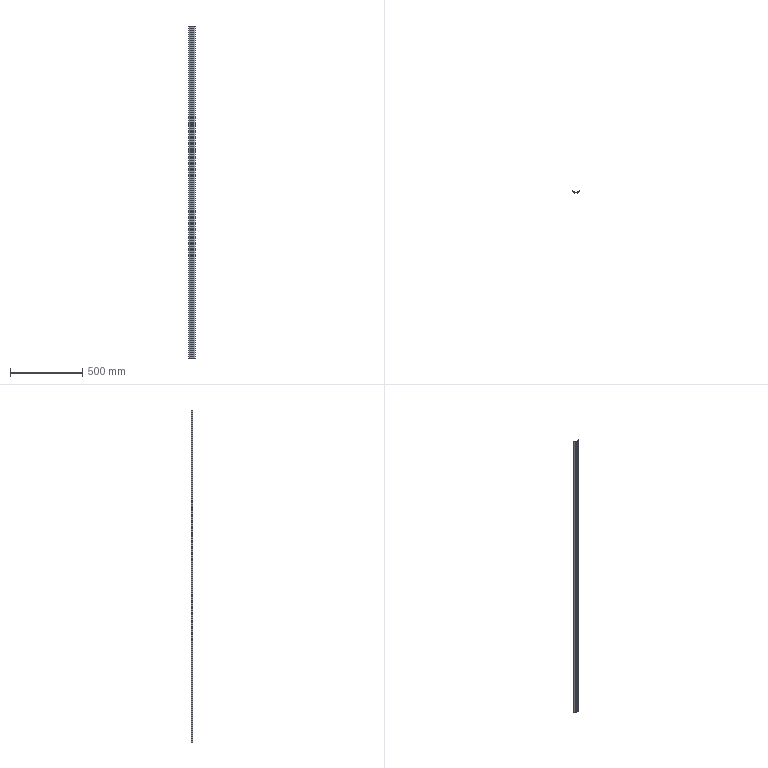Part | SolidWorks | features Extrusion 1 | 1 solid | 32 faces | box 46.782 x 13.535 x 2290 mm | volume 183913 mm3 | plane 25 | cylinder 7 | commonest cylinder face diameters 67.994 x4 0.2 x2 65.594 x1
STEP:
#1=CARTESIAN_POINT('',(-11.25,9.786,-1145.));
#2=VERTEX_POINT('',#1);
#3=CARTESIAN_POINT('',(-11.25,5.783,-1145.));
#4=VERTEX_POINT('',#3);
#5=CARTESIAN_POINT('',(-11.25,9.786,-1145.));
#6=DIRECTION('',(0.,-1.,0.));
#7=VECTOR('',#6,1000.);
#8=LINE('',#5,#7);
#9=EDGE_CURVE('',#2,#4,#8,.T.);
#10=ORIENTED_EDGE('',*,*,#9,.T.);
#11=CARTESIAN_POINT('',(-11.25,5.783,1145.));
#12=VERTEX_POINT('',#11);
#13=CARTESIAN_POINT('',(-11.25,5.783,1145.));
#14=DIRECTION('',(0.,0.,-1.));
#15=VECTOR('',#14,1000.);
#16=LINE('',#13,#15);
#17=EDGE_CURVE('',#12,#4,#16,.T.);
#18=ORIENTED_EDGE('',*,*,#17,.F.);
#19=CARTESIAN_POINT('',(-11.25,9.786,1145.));
#20=VERTEX_POINT('',#19);
#21=CARTESIAN_POINT('',(-11.25,9.786,1145.));
#22=DIRECTION('',(0.,-1.,0.));
#23=VECTOR('',#22,1000.);
#24=LINE('',#21,#23);
#25=EDGE_CURVE('',#20,#12,#24,.T.);
#26=ORIENTED_EDGE('',*,*,#25,.F.);
#27=CARTESIAN_POINT('',(-11.25,9.786,1145.));
#28=DIRECTION('',(0.,0.,-1.));
#29=VECTOR('',#28,1000.);
#30=LINE('',#27,#29);
#31=EDGE_CURVE('',#20,#2,#30,.T.);
#32=ORIENTED_EDGE('',*,*,#31,.T.);
#33=EDGE_LOOP('',(#10,#18,#26,#32));
#34=FACE_OUTER_BOUND('',#33,.T.);
#35=CARTESIAN_POINT('',(-11.25,9.786,1145.));
#36=DIRECTION('',(1.,0.,0.));
#37=DIRECTION('',(0.,0.,-1.));
#38=AXIS2_PLACEMENT_3D('',#35,#36,#37);
#39=PLANE('',#38);
#40=ADVANCED_FACE('',(#34),#39,.F.);
#41=CARTESIAN_POINT('',(-10.667,5.2,-1145.));
#42=VERTEX_POINT('',#41);
#43=CARTESIAN_POINT('',(-11.25,5.783,-1145.));
#44=DIRECTION('',(0.7071,-0.7071,0.));
#45=VECTOR('',#44,1000.);
#46=LINE('',#43,#45);
#47=EDGE_CURVE('',#4,#42,#46,.T.);
#48=ORIENTED_EDGE('',*,*,#47,.T.);
#49=CARTESIAN_POINT('',(-10.667,5.2,1145.));
#50=VERTEX_POINT('',#49);
#51=CARTESIAN_POINT('',(-10.667,5.2,1145.));
#52=DIRECTION('',(0.,0.,-1.));
#53=VECTOR('',#52,1000.);
#54=LINE('',#51,#53);
#55=EDGE_CURVE('',#50,#42,#54,.T.);
#56=ORIENTED_EDGE('',*,*,#55,.F.);
#57=CARTESIAN_POINT('',(-11.25,5.783,1145.));
#58=DIRECTION('',(0.7071,-0.7071,0.));
#59=VECTOR('',#58,1000.);
#60=LINE('',#57,#59);
#61=EDGE_CURVE('',#12,#50,#60,.T.);
#62=ORIENTED_EDGE('',*,*,#61,.F.);
#63=ORIENTED_EDGE('',*,*,#17,.T.);
#64=EDGE_LOOP('',(#48,#56,#62,#63));
#65=FACE_OUTER_BOUND('',#64,.T.);
#66=CARTESIAN_POINT('',(-11.25,5.783,1145.));
#67=DIRECTION('',(0.7071,0.7071,0.));
#68=DIRECTION('',(-0.7071,0.7071,0.));
#69=AXIS2_PLACEMENT_3D('',#66,#67,#68);
#70=PLANE('',#69);
#71=ADVANCED_FACE('',(#65),#70,.F.);
#72=CARTESIAN_POINT('',(-8.25,5.2,-1145.));
#73=VERTEX_POINT('',#72);
#74=CARTESIAN_POINT('',(-10.667,5.2,-1145.));
#75=DIRECTION('',(1.,0.,0.));
#76=VECTOR('',#75,1000.);
#77=LINE('',#74,#76);
#78=EDGE_CURVE('',#42,#73,#77,.T.);
#79=ORIENTED_EDGE('',*,*,#78,.T.);
#80=CARTESIAN_POINT('',(-8.25,5.2,1145.));
#81=VERTEX_POINT('',#80);
#82=CARTESIAN_POINT('',(-8.25,5.2,1145.));
#83=DIRECTION('',(0.,0.,-1.));
#84=VECTOR('',#83,1000.);
#85=LINE('',#82,#84);
#86=EDGE_CURVE('',#81,#73,#85,.T.);
#87=ORIENTED_EDGE('',*,*,#86,.F.);
#88=CARTESIAN_POINT('',(-10.667,5.2,1145.));
#89=DIRECTION('',(1.,0.,0.));
#90=VECTOR('',#89,1000.);
#91=LINE('',#88,#90);
#92=EDGE_CURVE('',#50,#81,#91,.T.);
#93=ORIENTED_EDGE('',*,*,#92,.F.);
#94=ORIENTED_EDGE('',*,*,#55,.T.);
#95=EDGE_LOOP('',(#79,#87,#93,#94));
#96=FACE_OUTER_BOUND('',#95,.T.);
#97=CARTESIAN_POINT('',(-10.667,5.2,1145.));
#98=DIRECTION('',(0.,1.,0.));
#99=DIRECTION('',(0.,0.,1.));
#100=AXIS2_PLACEMENT_3D('',#97,#98,#99);
#101=PLANE('',#100);
#102=ADVANCED_FACE('',(#96),#101,.F.);
#103=CARTESIAN_POINT('',(-8.25,6.,-1145.));
#104=VERTEX_POINT('',#103);
#105=CARTESIAN_POINT('',(-8.25,5.2,-1145.));
#106=DIRECTION('',(0.,1.,0.));
#107=VECTOR('',#106,1000.);
#108=LINE('',#105,#107);
#109=EDGE_CURVE('',#73,#104,#108,.T.);
#110=ORIENTED_EDGE('',*,*,#109,.T.);
#111=CARTESIAN_POINT('',(-8.25,6.,1145.));
#112=VERTEX_POINT('',#111);
#113=CARTESIAN_POINT('',(-8.25,6.,1145.));
#114=DIRECTION('',(0.,0.,-1.));
#115=VECTOR('',#114,1000.);
#116=LINE('',#113,#115);
#117=EDGE_CURVE('',#112,#104,#116,.T.);
#118=ORIENTED_EDGE('',*,*,#117,.F.);
#119=CARTESIAN_POINT('',(-8.25,5.2,1145.));
#120=DIRECTION('',(0.,1.,0.));
#121=VECTOR('',#120,1000.);
#122=LINE('',#119,#121);
#123=EDGE_CURVE('',#81,#112,#122,.T.);
#124=ORIENTED_EDGE('',*,*,#123,.F.);
#125=ORIENTED_EDGE('',*,*,#86,.T.);
#126=EDGE_LOOP('',(#110,#118,#124,#125));
#127=FACE_OUTER_BOUND('',#126,.T.);
#128=CARTESIAN_POINT('',(-8.25,5.2,1145.));
#129=DIRECTION('',(-1.,0.,0.));
#130=DIRECTION('',(0.,0.,1.));
#131=AXIS2_PLACEMENT_3D('',#128,#129,#130);
#132=PLANE('',#131);
#133=ADVANCED_FACE('',(#127),#132,.F.);
#134=CARTESIAN_POINT('',(-10.25,6.,-1145.));
#135=VERTEX_POINT('',#134);
#136=CARTESIAN_POINT('',(-8.25,6.,-1145.));
#137=DIRECTION('',(-1.,0.,0.));
#138=VECTOR('',#137,1000.);
#139=LINE('',#136,#138);
#140=EDGE_CURVE('',#104,#135,#139,.T.);
#141=ORIENTED_EDGE('',*,*,#140,.T.);
#142=CARTESIAN_POINT('',(-10.25,6.,1145.));
#143=VERTEX_POINT('',#142);
#144=CARTESIAN_POINT('',(-10.25,6.,1145.));
#145=DIRECTION('',(0.,0.,-1.));
#146=VECTOR('',#145,1000.);
#147=LINE('',#144,#146);
#148=EDGE_CURVE('',#143,#135,#147,.T.);
#149=ORIENTED_EDGE('',*,*,#148,.F.);
#150=CARTESIAN_POINT('',(-8.25,6.,1145.));
#151=DIRECTION('',(-1.,0.,0.));
#152=VECTOR('',#151,1000.);
#153=LINE('',#150,#152);
#154=EDGE_CURVE('',#112,#143,#153,.T.);
#155=ORIENTED_EDGE('',*,*,#154,.F.);
#156=ORIENTED_EDGE('',*,*,#117,.T.);
#157=EDGE_LOOP('',(#141,#149,#155,#156));
#158=FACE_OUTER_BOUND('',#157,.T.);
#159=CARTESIAN_POINT('',(-8.25,6.,1145.));
#160=DIRECTION('',(0.,-1.,0.));
#161=DIRECTION('',(0.,0.,-1.));
#162=AXIS2_PLACEMENT_3D('',#159,#160,#161);
#163=PLANE('',#162);
#164=ADVANCED_FACE('',(#158),#163,.F.);
#165=CARTESIAN_POINT('',(-10.25,7.726,-1145.));
#166=VERTEX_POINT('',#165);
#167=CARTESIAN_POINT('',(-10.25,6.,-1145.));
#168=DIRECTION('',(0.,1.,0.));
#169=VECTOR('',#168,1000.);
#170=LINE('',#167,#169);
#171=EDGE_CURVE('',#135,#166,#170,.T.);
#172=ORIENTED_EDGE('',*,*,#171,.T.);
#173=CARTESIAN_POINT('',(-10.25,7.726,1145.));
#174=VERTEX_POINT('',#173);
#175=CARTESIAN_POINT('',(-10.25,7.726,1145.));
#176=DIRECTION('',(0.,0.,-1.));
#177=VECTOR('',#176,1000.);
#178=LINE('',#175,#177);
#179=EDGE_CURVE('',#174,#166,#178,.T.);
#180=ORIENTED_EDGE('',*,*,#179,.F.);
#181=CARTESIAN_POINT('',(-10.25,6.,1145.));
#182=DIRECTION('',(0.,1.,0.));
#183=VECTOR('',#182,1000.);
#184=LINE('',#181,#183);
#185=EDGE_CURVE('',#143,#174,#184,.T.);
#186=ORIENTED_EDGE('',*,*,#185,.F.);
#187=ORIENTED_EDGE('',*,*,#148,.T.);
#188=EDGE_LOOP('',(#172,#180,#186,#187));
#189=FACE_OUTER_BOUND('',#188,.T.);
#190=CARTESIAN_POINT('',(-10.25,6.,1145.));
#191=DIRECTION('',(-1.,0.,0.));
#192=DIRECTION('',(0.,0.,1.));
#193=AXIS2_PLACEMENT_3D('',#190,#191,#192);
#194=PLANE('',#193);
#195=ADVANCED_FACE('',(#189),#194,.F.);
#196=CARTESIAN_POINT('',(-9.,7.725,-1145.));
#197=VERTEX_POINT('',#196);
#198=CARTESIAN_POINT('',(-10.25,7.726,-1145.));
#199=DIRECTION('',(1.,-0.001291,0.));
#200=VECTOR('',#199,1000.);
#201=LINE('',#198,#200);
#202=EDGE_CURVE('',#166,#197,#201,.T.);
#203=ORIENTED_EDGE('',*,*,#202,.T.);
#204=CARTESIAN_POINT('',(-9.,7.725,1145.));
#205=VERTEX_POINT('',#204);
#206=CARTESIAN_POINT('',(-9.,7.725,1145.));
#207=DIRECTION('',(0.,0.,-1.));
#208=VECTOR('',#207,1000.);
#209=LINE('',#206,#208);
#210=EDGE_CURVE('',#205,#197,#209,.T.);
#211=ORIENTED_EDGE('',*,*,#210,.F.);
#212=CARTESIAN_POINT('',(-10.25,7.726,1145.));
#213=DIRECTION('',(1.,-0.001291,0.));
#214=VECTOR('',#213,1000.);
#215=LINE('',#212,#214);
#216=EDGE_CURVE('',#174,#205,#215,.T.);
#217=ORIENTED_EDGE('',*,*,#216,.F.);
#218=ORIENTED_EDGE('',*,*,#179,.T.);
#219=EDGE_LOOP('',(#203,#211,#217,#218));
#220=FACE_OUTER_BOUND('',#219,.T.);
#221=CARTESIAN_POINT('',(-10.25,7.726,1145.));
#222=DIRECTION('',(0.001291,1.,0.));
#223=DIRECTION('',(-1.,0.001291,0.));
#224=AXIS2_PLACEMENT_3D('',#221,#222,#223);
#225=PLANE('',#224);
#226=ADVANCED_FACE('',(#220),#225,.F.);
#227=CARTESIAN_POINT('',(-8.25,8.474,-1145.));
#228=VERTEX_POINT('',#227);
#229=CARTESIAN_POINT('',(-9.,7.725,-1145.));
#230=DIRECTION('',(0.7076,0.7067,0.));
#231=VECTOR('',#230,1000.);
#232=LINE('',#229,#231);
#233=EDGE_CURVE('',#197,#228,#232,.T.);
#234=ORIENTED_EDGE('',*,*,#233,.T.);
#235=CARTESIAN_POINT('',(-8.25,8.474,1145.));
#236=VERTEX_POINT('',#235);
#237=CARTESIAN_POINT('',(-8.25,8.474,1145.));
#238=DIRECTION('',(0.,0.,-1.));
#239=VECTOR('',#238,1000.);
#240=LINE('',#237,#239);
#241=EDGE_CURVE('',#236,#228,#240,.T.);
#242=ORIENTED_EDGE('',*,*,#241,.F.);
#243=CARTESIAN_POINT('',(-9.,7.725,1145.));
#244=DIRECTION('',(0.7076,0.7067,0.));
#245=VECTOR('',#244,1000.);
#246=LINE('',#243,#245);
#247=EDGE_CURVE('',#205,#236,#246,.T.);
#248=ORIENTED_EDGE('',*,*,#247,.F.);
#249=ORIENTED_EDGE('',*,*,#210,.T.);
#250=EDGE_LOOP('',(#234,#242,#248,#249));
#251=FACE_OUTER_BOUND('',#250,.T.);
#252=CARTESIAN_POINT('',(-9.,7.725,1145.));
#253=DIRECTION('',(-0.7067,0.7076,0.));
#254=DIRECTION('',(-0.7076,-0.7067,0.));
#255=AXIS2_PLACEMENT_3D('',#252,#253,#254);
#256=PLANE('',#255);
#257=ADVANCED_FACE('',(#251),#256,.F.);
#258=CARTESIAN_POINT('',(-8.25,8.887,-1145.));
#259=VERTEX_POINT('',#258);
#260=CARTESIAN_POINT('',(-8.25,8.474,-1145.));
#261=DIRECTION('',(0.,1.,0.));
#262=VECTOR('',#261,1000.);
#263=LINE('',#260,#262);
#264=EDGE_CURVE('',#228,#259,#263,.T.);
#265=ORIENTED_EDGE('',*,*,#264,.T.);
#266=CARTESIAN_POINT('',(-8.25,8.887,1145.));
#267=VERTEX_POINT('',#266);
#268=CARTESIAN_POINT('',(-8.25,8.887,1145.));
#269=DIRECTION('',(0.,0.,-1.));
#270=VECTOR('',#269,1000.);
#271=LINE('',#268,#270);
#272=EDGE_CURVE('',#267,#259,#271,.T.);
#273=ORIENTED_EDGE('',*,*,#272,.F.);
#274=CARTESIAN_POINT('',(-8.25,8.474,1145.));
#275=DIRECTION('',(0.,1.,0.));
#276=VECTOR('',#275,1000.);
#277=LINE('',#274,#276);
#278=EDGE_CURVE('',#236,#267,#277,.T.);
#279=ORIENTED_EDGE('',*,*,#278,.F.);
#280=ORIENTED_EDGE('',*,*,#241,.T.);
#281=EDGE_LOOP('',(#265,#273,#279,#280));
#282=FACE_OUTER_BOUND('',#281,.T.);
#283=CARTESIAN_POINT('',(-8.25,8.474,1145.));
#284=DIRECTION('',(-1.,0.,0.));
#285=DIRECTION('',(0.,0.,1.));
#286=AXIS2_PLACEMENT_3D('',#283,#284,#285);
#287=PLANE('',#286);
#288=ADVANCED_FACE('',(#282),#287,.F.);
#289=CARTESIAN_POINT('',(-3.,8.003,-1145.));
#290=VERTEX_POINT('',#289);
#291=CARTESIAN_POINT('',(0.,41.867,-1145.));
#292=DIRECTION('',(0.,0.,1.));
#293=DIRECTION('',(1.,0.,0.));
#294=AXIS2_PLACEMENT_3D('',#291,#292,#293);
#295=CIRCLE('',#294,33.997);
#296=EDGE_CURVE('',#259,#290,#295,.T.);
#297=ORIENTED_EDGE('',*,*,#296,.T.);
#298=CARTESIAN_POINT('',(-3.,8.003,1145.));
#299=VERTEX_POINT('',#298);
#300=CARTESIAN_POINT('',(-3.,8.003,1145.));
#301=DIRECTION('',(0.,0.,-1.));
#302=VECTOR('',#301,1000.);
#303=LINE('',#300,#302);
#304=EDGE_CURVE('',#299,#290,#303,.T.);
#305=ORIENTED_EDGE('',*,*,#304,.F.);
#306=CARTESIAN_POINT('',(0.,41.867,1145.));
#307=DIRECTION('',(0.,0.,1.));
#308=DIRECTION('',(1.,0.,0.));
#309=AXIS2_PLACEMENT_3D('',#306,#307,#308);
#310=CIRCLE('',#309,33.997);
#311=EDGE_CURVE('',#267,#299,#310,.T.);
#312=ORIENTED_EDGE('',*,*,#311,.F.);
#313=ORIENTED_EDGE('',*,*,#272,.T.);
#314=EDGE_LOOP('',(#297,#305,#312,#313));
#315=FACE_OUTER_BOUND('',#314,.T.);
#316=CARTESIAN_POINT('',(0.,41.867,1145.));
#317=DIRECTION('',(0.,0.,-1.));
#318=DIRECTION('',(-1.,0.,0.));
#319=AXIS2_PLACEMENT_3D('',#316,#317,#318);
#320=CYLINDRICAL_SURFACE('',#319,33.997);
#321=ADVANCED_FACE('',(#315),#320,.T.);
#322=CARTESIAN_POINT('',(-3.,7.702,-1145.));
#323=VERTEX_POINT('',#322);
#324=CARTESIAN_POINT('',(-3.,8.003,-1145.));
#325=DIRECTION('',(0.,-1.,0.));
#326=VECTOR('',#325,1000.);
#327=LINE('',#324,#326);
#328=EDGE_CURVE('',#290,#323,#327,.T.);
#329=ORIENTED_EDGE('',*,*,#328,.T.);
#330=CARTESIAN_POINT('',(-3.,7.702,1145.));
#331=VERTEX_POINT('',#330);
#332=CARTESIAN_POINT('',(-3.,7.702,1145.));
#333=DIRECTION('',(0.,0.,-1.));
#334=VECTOR('',#333,1000.);
#335=LINE('',#332,#334);
#336=EDGE_CURVE('',#331,#323,#335,.T.);
#337=ORIENTED_EDGE('',*,*,#336,.F.);
#338=CARTESIAN_POINT('',(-3.,8.003,1145.));
#339=DIRECTION('',(0.,-1.,0.));
#340=VECTOR('',#339,1000.);
#341=LINE('',#338,#340);
#342=EDGE_CURVE('',#299,#331,#341,.T.);
#343=ORIENTED_EDGE('',*,*,#342,.F.);
#344=ORIENTED_EDGE('',*,*,#304,.T.);
#345=EDGE_LOOP('',(#329,#337,#343,#344));
#346=FACE_OUTER_BOUND('',#345,.T.);
#347=CARTESIAN_POINT('',(-3.,8.003,1145.));
#348=DIRECTION('',(1.,0.,0.));
#349=DIRECTION('',(0.,0.,-1.));
#350=AXIS2_PLACEMENT_3D('',#347,#348,#349);
#351=PLANE('',#350);
#352=ADVANCED_FACE('',(#346),#351,.F.);
#353=CARTESIAN_POINT('',(3.,7.702,-1145.));
#354=VERTEX_POINT('',#353);
#355=CARTESIAN_POINT('',(-3.,7.702,-1145.));
#356=DIRECTION('',(1.,0.,0.));
#357=VECTOR('',#356,1000.);
#358=LINE('',#355,#357);
#359=EDGE_CURVE('',#323,#354,#358,.T.);
#360=ORIENTED_EDGE('',*,*,#359,.T.);
#361=CARTESIAN_POINT('',(3.,7.702,1145.));
#362=VERTEX_POINT('',#361);
#363=CARTESIAN_POINT('',(3.,7.702,1145.));
#364=DIRECTION('',(0.,0.,-1.));
#365=VECTOR('',#364,1000.);
#366=LINE('',#363,#365);
#367=EDGE_CURVE('',#362,#354,#366,.T.);
#368=ORIENTED_EDGE('',*,*,#367,.F.);
#369=CARTESIAN_POINT('',(-3.,7.702,1145.));
#370=DIRECTION('',(1.,0.,0.));
#371=VECTOR('',#370,1000.);
#372=LINE('',#369,#371);
#373=EDGE_CURVE('',#331,#362,#372,.T.);
#374=ORIENTED_EDGE('',*,*,#373,.F.);
#375=ORIENTED_EDGE('',*,*,#336,.T.);
#376=EDGE_LOOP('',(#360,#368,#374,#375));
#377=FACE_OUTER_BOUND('',#376,.T.);
#378=CARTESIAN_POINT('',(-3.,7.702,1145.));
#379=DIRECTION('',(0.,1.,0.));
#380=DIRECTION('',(0.,0.,1.));
#381=AXIS2_PLACEMENT_3D('',#378,#379,#380);
#382=PLANE('',#381);
#383=ADVANCED_FACE('',(#377),#382,.F.);
#384=CARTESIAN_POINT('',(3.,8.003,-1145.));
#385=VERTEX_POINT('',#384);
#386=CARTESIAN_POINT('',(3.,7.702,-1145.));
#387=DIRECTION('',(0.,1.,0.));
#388=VECTOR('',#387,1000.);
#389=LINE('',#386,#388);
#390=EDGE_CURVE('',#354,#385,#389,.T.);
#391=ORIENTED_EDGE('',*,*,#390,.T.);
#392=CARTESIAN_POINT('',(3.,8.003,1145.));
#393=VERTEX_POINT('',#392);
#394=CARTESIAN_POINT('',(3.,8.003,1145.));
#395=DIRECTION('',(0.,0.,-1.));
#396=VECTOR('',#395,1000.);
#397=LINE('',#394,#396);
#398=EDGE_CURVE('',#393,#385,#397,.T.);
#399=ORIENTED_EDGE('',*,*,#398,.F.);
#400=CARTESIAN_POINT('',(3.,7.702,1145.));
#401=DIRECTION('',(0.,1.,0.));
#402=VECTOR('',#401,1000.);
#403=LINE('',#400,#402);
#404=EDGE_CURVE('',#362,#393,#403,.T.);
#405=ORIENTED_EDGE('',*,*,#404,.F.);
#406=ORIENTED_EDGE('',*,*,#367,.T.);
#407=EDGE_LOOP('',(#391,#399,#405,#406));
#408=FACE_OUTER_BOUND('',#407,.T.);
#409=CARTESIAN_POINT('',(3.,7.702,1145.));
#410=DIRECTION('',(-1.,0.,0.));
#411=DIRECTION('',(0.,0.,1.));
#412=AXIS2_PLACEMENT_3D('',#409,#410,#411);
#413=PLANE('',#412);
#414=ADVANCED_FACE('',(#408),#413,.F.);
#415=CARTESIAN_POINT('',(8.25,8.887,-1145.));
#416=VERTEX_POINT('',#415);
#417=CARTESIAN_POINT('',(0.,41.867,-1145.));
#418=DIRECTION('',(0.,0.,1.));
#419=DIRECTION('',(1.,0.,0.));
#420=AXIS2_PLACEMENT_3D('',#417,#418,#419);
#421=CIRCLE('',#420,33.997);
#422=EDGE_CURVE('',#385,#416,#421,.T.);
#423=ORIENTED_EDGE('',*,*,#422,.T.);
#424=CARTESIAN_POINT('',(8.25,8.887,1145.));
#425=VERTEX_POINT('',#424);
#426=CARTESIAN_POINT('',(8.25,8.887,1145.));
#427=DIRECTION('',(0.,0.,-1.));
#428=VECTOR('',#427,1000.);
#429=LINE('',#426,#428);
#430=EDGE_CURVE('',#425,#416,#429,.T.);
#431=ORIENTED_EDGE('',*,*,#430,.F.);
#432=CARTESIAN_POINT('',(0.,41.867,1145.));
#433=DIRECTION('',(0.,0.,1.));
#434=DIRECTION('',(1.,0.,0.));
#435=AXIS2_PLACEMENT_3D('',#432,#433,#434);
#436=CIRCLE('',#435,33.997);
#437=EDGE_CURVE('',#393,#425,#436,.T.);
#438=ORIENTED_EDGE('',*,*,#437,.F.);
#439=ORIENTED_EDGE('',*,*,#398,.T.);
#440=EDGE_LOOP('',(#423,#431,#438,#439));
#441=FACE_OUTER_BOUND('',#440,.T.);
#442=CARTESIAN_POINT('',(0.,41.867,1145.));
#443=DIRECTION('',(0.,0.,-1.));
#444=DIRECTION('',(-1.,0.,0.));
#445=AXIS2_PLACEMENT_3D('',#442,#443,#444);
#446=CYLINDRICAL_SURFACE('',#445,33.997);
#447=ADVANCED_FACE('',(#441),#446,.T.);
#448=CARTESIAN_POINT('',(8.25,8.474,-1145.));
#449=VERTEX_POINT('',#448);
#450=CARTESIAN_POINT('',(8.25,8.887,-1145.));
#451=DIRECTION('',(0.,-1.,0.));
#452=VECTOR('',#451,1000.);
#453=LINE('',#450,#452);
#454=EDGE_CURVE('',#416,#449,#453,.T.);
#455=ORIENTED_EDGE('',*,*,#454,.T.);
#456=CARTESIAN_POINT('',(8.25,8.474,1145.));
#457=VERTEX_POINT('',#456);
#458=CARTESIAN_POINT('',(8.25,8.474,1145.));
#459=DIRECTION('',(0.,0.,-1.));
#460=VECTOR('',#459,1000.);
#461=LINE('',#458,#460);
#462=EDGE_CURVE('',#457,#449,#461,.T.);
#463=ORIENTED_EDGE('',*,*,#462,.F.);
#464=CARTESIAN_POINT('',(8.25,8.887,1145.));
#465=DIRECTION('',(0.,-1.,0.));
#466=VECTOR('',#465,1000.);
#467=LINE('',#464,#466);
#468=EDGE_CURVE('',#425,#457,#467,.T.);
#469=ORIENTED_EDGE('',*,*,#468,.F.);
#470=ORIENTED_EDGE('',*,*,#430,.T.);
#471=EDGE_LOOP('',(#455,#463,#469,#470));
#472=FACE_OUTER_BOUND('',#471,.T.);
#473=CARTESIAN_POINT('',(8.25,8.887,1145.));
#474=DIRECTION('',(1.,0.,0.));
#475=DIRECTION('',(0.,0.,-1.));
#476=AXIS2_PLACEMENT_3D('',#473,#474,#475);
#477=PLANE('',#476);
#478=ADVANCED_FACE('',(#472),#477,.F.);
#479=CARTESIAN_POINT('',(9.,7.725,-1145.));
#480=VERTEX_POINT('',#479);
#481=CARTESIAN_POINT('',(8.25,8.474,-1145.));
#482=DIRECTION('',(0.7076,-0.7067,0.));
#483=VECTOR('',#482,1000.);
#484=LINE('',#481,#483);
#485=EDGE_CURVE('',#449,#480,#484,.T.);
#486=ORIENTED_EDGE('',*,*,#485,.T.);
#487=CARTESIAN_POINT('',(9.,7.725,1145.));
#488=VERTEX_POINT('',#487);
#489=CARTESIAN_POINT('',(9.,7.725,1145.));
#490=DIRECTION('',(0.,0.,-1.));
#491=VECTOR('',#490,1000.);
#492=LINE('',#489,#491);
#493=EDGE_CURVE('',#488,#480,#492,.T.);
#494=ORIENTED_EDGE('',*,*,#493,.F.);
#495=CARTESIAN_POINT('',(8.25,8.474,1145.));
#496=DIRECTION('',(0.7076,-0.7067,0.));
#497=VECTOR('',#496,1000.);
#498=LINE('',#495,#497);
#499=EDGE_CURVE('',#457,#488,#498,.T.);
#500=ORIENTED_EDGE('',*,*,#499,.F.);
#501=ORIENTED_EDGE('',*,*,#462,.T.);
#502=EDGE_LOOP('',(#486,#494,#500,#501));
#503=FACE_OUTER_BOUND('',#502,.T.);
#504=CARTESIAN_POINT('',(8.25,8.474,1145.));
#505=DIRECTION('',(0.7067,0.7076,0.));
#506=DIRECTION('',(-0.7076,0.7067,0.));
#507=AXIS2_PLACEMENT_3D('',#504,#505,#506);
#508=PLANE('',#507);
#509=ADVANCED_FACE('',(#503),#508,.F.);
#510=CARTESIAN_POINT('',(10.25,7.726,-1145.));
#511=VERTEX_POINT('',#510);
#512=CARTESIAN_POINT('',(9.,7.725,-1145.));
#513=DIRECTION('',(1.,0.001291,0.));
#514=VECTOR('',#513,1000.);
#515=LINE('',#512,#514);
#516=EDGE_CURVE('',#480,#511,#515,.T.);
#517=ORIENTED_EDGE('',*,*,#516,.T.);
#518=CARTESIAN_POINT('',(10.25,7.726,1145.));
#519=VERTEX_POINT('',#518);
#520=CARTESIAN_POINT('',(10.25,7.726,1145.));
#521=DIRECTION('',(0.,0.,-1.));
#522=VECTOR('',#521,1000.);
#523=LINE('',#520,#522);
#524=EDGE_CURVE('',#519,#511,#523,.T.);
#525=ORIENTED_EDGE('',*,*,#524,.F.);
#526=CARTESIAN_POINT('',(9.,7.725,1145.));
#527=DIRECTION('',(1.,0.001291,0.));
#528=VECTOR('',#527,1000.);
#529=LINE('',#526,#528);
#530=EDGE_CURVE('',#488,#519,#529,.T.);
#531=ORIENTED_EDGE('',*,*,#530,.F.);
#532=ORIENTED_EDGE('',*,*,#493,.T.);
#533=EDGE_LOOP('',(#517,#525,#531,#532));
#534=FACE_OUTER_BOUND('',#533,.T.);
#535=CARTESIAN_POINT('',(9.,7.725,1145.));
#536=DIRECTION('',(-0.001291,1.,0.));
#537=DIRECTION('',(-1.,-0.001291,0.));
#538=AXIS2_PLACEMENT_3D('',#535,#536,#537);
#539=PLANE('',#538);
#540=ADVANCED_FACE('',(#534),#539,.F.);
#541=CARTESIAN_POINT('',(10.25,6.,-1145.));
#542=VERTEX_POINT('',#541);
#543=CARTESIAN_POINT('',(10.25,7.726,-1145.));
#544=DIRECTION('',(0.,-1.,0.));
#545=VECTOR('',#544,1000.);
#546=LINE('',#543,#545);
#547=EDGE_CURVE('',#511,#542,#546,.T.);
#548=ORIENTED_EDGE('',*,*,#547,.T.);
#549=CARTESIAN_POINT('',(10.25,6.,1145.));
#550=VERTEX_POINT('',#549);
#551=CARTESIAN_POINT('',(10.25,6.,1145.));
#552=DIRECTION('',(0.,0.,-1.));
#553=VECTOR('',#552,1000.);
#554=LINE('',#551,#553);
#555=EDGE_CURVE('',#550,#542,#554,.T.);
#556=ORIENTED_EDGE('',*,*,#555,.F.);
#557=CARTESIAN_POINT('',(10.25,7.726,1145.));
#558=DIRECTION('',(0.,-1.,0.));
#559=VECTOR('',#558,1000.);
#560=LINE('',#557,#559);
#561=EDGE_CURVE('',#519,#550,#560,.T.);
#562=ORIENTED_EDGE('',*,*,#561,.F.);
#563=ORIENTED_EDGE('',*,*,#524,.T.);
#564=EDGE_LOOP('',(#548,#556,#562,#563));
#565=FACE_OUTER_BOUND('',#564,.T.);
#566=CARTESIAN_POINT('',(10.25,7.726,1145.));
#567=DIRECTION('',(1.,0.,0.));
#568=DIRECTION('',(0.,0.,-1.));
#569=AXIS2_PLACEMENT_3D('',#566,#567,#568);
#570=PLANE('',#569);
#571=ADVANCED_FACE('',(#565),#570,.F.);
#572=CARTESIAN_POINT('',(8.25,6.,-1145.));
#573=VERTEX_POINT('',#572);
#574=CARTESIAN_POINT('',(10.25,6.,-1145.));
#575=DIRECTION('',(-1.,0.,0.));
#576=VECTOR('',#575,1000.);
#577=LINE('',#574,#576);
#578=EDGE_CURVE('',#542,#573,#577,.T.);
#579=ORIENTED_EDGE('',*,*,#578,.T.);
#580=CARTESIAN_POINT('',(8.25,6.,1145.));
#581=VERTEX_POINT('',#580);
#582=CARTESIAN_POINT('',(8.25,6.,1145.));
#583=DIRECTION('',(0.,0.,-1.));
#584=VECTOR('',#583,1000.);
#585=LINE('',#582,#584);
#586=EDGE_CURVE('',#581,#573,#585,.T.);
#587=ORIENTED_EDGE('',*,*,#586,.F.);
#588=CARTESIAN_POINT('',(10.25,6.,1145.));
#589=DIRECTION('',(-1.,0.,0.));
#590=VECTOR('',#589,1000.);
#591=LINE('',#588,#590);
#592=EDGE_CURVE('',#550,#581,#591,.T.);
#593=ORIENTED_EDGE('',*,*,#592,.F.);
#594=ORIENTED_EDGE('',*,*,#555,.T.);
#595=EDGE_LOOP('',(#579,#587,#593,#594));
#596=FACE_OUTER_BOUND('',#595,.T.);
#597=CARTESIAN_POINT('',(10.25,6.,1145.));
#598=DIRECTION('',(0.,-1.,0.));
#599=DIRECTION('',(0.,0.,-1.));
#600=AXIS2_PLACEMENT_3D('',#597,#598,#599);
#601=PLANE('',#600);
#602=ADVANCED_FACE('',(#596),#601,.F.);
#603=CARTESIAN_POINT('',(8.25,5.2,-1145.));
#604=VERTEX_POINT('',#603);
#605=CARTESIAN_POINT('',(8.25,6.,-1145.));
#606=DIRECTION('',(0.,-1.,0.));
#607=VECTOR('',#606,1000.);
#608=LINE('',#605,#607);
#609=EDGE_CURVE('',#573,#604,#608,.T.);
#610=ORIENTED_EDGE('',*,*,#609,.T.);
#611=CARTESIAN_POINT('',(8.25,5.2,1145.));
#612=VERTEX_POINT('',#611);
#613=CARTESIAN_POINT('',(8.25,5.2,1145.));
#614=DIRECTION('',(0.,0.,-1.));
#615=VECTOR('',#614,1000.);
#616=LINE('',#613,#615);
#617=EDGE_CURVE('',#612,#604,#616,.T.);
#618=ORIENTED_EDGE('',*,*,#617,.F.);
#619=CARTESIAN_POINT('',(8.25,6.,1145.));
#620=DIRECTION('',(0.,-1.,0.));
#621=VECTOR('',#620,1000.);
#622=LINE('',#619,#621);
#623=EDGE_CURVE('',#581,#612,#622,.T.);
#624=ORIENTED_EDGE('',*,*,#623,.F.);
#625=ORIENTED_EDGE('',*,*,#586,.T.);
#626=EDGE_LOOP('',(#610,#618,#624,#625));
#627=FACE_OUTER_BOUND('',#626,.T.);
#628=CARTESIAN_POINT('',(8.25,6.,1145.));
#629=DIRECTION('',(1.,0.,0.));
#630=DIRECTION('',(0.,0.,-1.));
#631=AXIS2_PLACEMENT_3D('',#628,#629,#630);
#632=PLANE('',#631);
#633=ADVANCED_FACE('',(#627),#632,.F.);
#634=CARTESIAN_POINT('',(10.667,5.2,-1145.));
#635=VERTEX_POINT('',#634);
#636=CARTESIAN_POINT('',(8.25,5.2,-1145.));
#637=DIRECTION('',(1.,0.,0.));
#638=VECTOR('',#637,1000.);
#639=LINE('',#636,#638);
#640=EDGE_CURVE('',#604,#635,#639,.T.);
#641=ORIENTED_EDGE('',*,*,#640,.T.);
#642=CARTESIAN_POINT('',(10.667,5.2,1145.));
#643=VERTEX_POINT('',#642);
#644=CARTESIAN_POINT('',(10.667,5.2,1145.));
#645=DIRECTION('',(0.,0.,-1.));
#646=VECTOR('',#645,1000.);
#647=LINE('',#644,#646);
#648=EDGE_CURVE('',#643,#635,#647,.T.);
#649=ORIENTED_EDGE('',*,*,#648,.F.);
#650=CARTESIAN_POINT('',(8.25,5.2,1145.));
#651=DIRECTION('',(1.,0.,0.));
#652=VECTOR('',#651,1000.);
#653=LINE('',#650,#652);
#654=EDGE_CURVE('',#612,#643,#653,.T.);
#655=ORIENTED_EDGE('',*,*,#654,.F.);
#656=ORIENTED_EDGE('',*,*,#617,.T.);
#657=EDGE_LOOP('',(#641,#649,#655,#656));
#658=FACE_OUTER_BOUND('',#657,.T.);
#659=CARTESIAN_POINT('',(8.25,5.2,1145.));
#660=DIRECTION('',(0.,1.,0.));
#661=DIRECTION('',(0.,0.,1.));
#662=AXIS2_PLACEMENT_3D('',#659,#660,#661);
#663=PLANE('',#662);
#664=ADVANCED_FACE('',(#658),#663,.F.);
#665=CARTESIAN_POINT('',(11.25,5.783,-1145.));
#666=VERTEX_POINT('',#665);
#667=CARTESIAN_POINT('',(10.667,5.2,-1145.));
#668=DIRECTION('',(0.7071,0.7071,0.));
#669=VECTOR('',#668,1000.);
#670=LINE('',#667,#669);
#671=EDGE_CURVE('',#635,#666,#670,.T.);
#672=ORIENTED_EDGE('',*,*,#671,.T.);
#673=CARTESIAN_POINT('',(11.25,5.783,1145.));
#674=VERTEX_POINT('',#673);
#675=CARTESIAN_POINT('',(11.25,5.783,1145.));
#676=DIRECTION('',(0.,0.,-1.));
#677=VECTOR('',#676,1000.);
#678=LINE('',#675,#677);
#679=EDGE_CURVE('',#674,#666,#678,.T.);
#680=ORIENTED_EDGE('',*,*,#679,.F.);
#681=CARTESIAN_POINT('',(10.667,5.2,1145.));
#682=DIRECTION('',(0.7071,0.7071,0.));
#683=VECTOR('',#682,1000.);
#684=LINE('',#681,#683);
#685=EDGE_CURVE('',#643,#674,#684,.T.);
#686=ORIENTED_EDGE('',*,*,#685,.F.);
#687=ORIENTED_EDGE('',*,*,#648,.T.);
#688=EDGE_LOOP('',(#672,#680,#686,#687));
#689=FACE_OUTER_BOUND('',#688,.T.);
#690=CARTESIAN_POINT('',(10.667,5.2,1145.));
#691=DIRECTION('',(-0.7071,0.7071,0.));
#692=DIRECTION('',(-0.7071,-0.7071,0.));
#693=AXIS2_PLACEMENT_3D('',#690,#691,#692);
#694=PLANE('',#693);
#695=ADVANCED_FACE('',(#689),#694,.F.);
#696=CARTESIAN_POINT('',(11.25,9.786,-1145.));
#697=VERTEX_POINT('',#696);
#698=CARTESIAN_POINT('',(11.25,5.783,-1145.));
#699=DIRECTION('',(0.,1.,0.));
#700=VECTOR('',#699,1000.);
#701=LINE('',#698,#700);
#702=EDGE_CURVE('',#666,#697,#701,.T.);
#703=ORIENTED_EDGE('',*,*,#702,.T.);
#704=CARTESIAN_POINT('',(11.25,9.786,1145.));
#705=VERTEX_POINT('',#704);
#706=CARTESIAN_POINT('',(11.25,9.786,1145.));
#707=DIRECTION('',(0.,0.,-1.));
#708=VECTOR('',#707,1000.);
#709=LINE('',#706,#708);
#710=EDGE_CURVE('',#705,#697,#709,.T.);
#711=ORIENTED_EDGE('',*,*,#710,.F.);
#712=CARTESIAN_POINT('',(11.25,5.783,1145.));
#713=DIRECTION('',(0.,1.,0.));
#714=VECTOR('',#713,1000.);
#715=LINE('',#712,#714);
#716=EDGE_CURVE('',#674,#705,#715,.T.);
#717=ORIENTED_EDGE('',*,*,#716,.F.);
#718=ORIENTED_EDGE('',*,*,#679,.T.);
#719=EDGE_LOOP('',(#703,#711,#717,#718));
#720=FACE_OUTER_BOUND('',#719,.T.);
#721=CARTESIAN_POINT('',(11.25,5.783,1145.));
#722=DIRECTION('',(-1.,0.,0.));
#723=DIRECTION('',(0.,0.,1.));
#724=AXIS2_PLACEMENT_3D('',#721,#722,#723);
#725=PLANE('',#724);
#726=ADVANCED_FACE('',(#720),#725,.F.);
#727=CARTESIAN_POINT('',(23.391,17.196,-1145.));
#728=VERTEX_POINT('',#727);
#729=CARTESIAN_POINT('',(0.,41.867,-1145.));
#730=DIRECTION('',(0.,0.,1.));
#731=DIRECTION('',(1.,0.,0.));
#732=AXIS2_PLACEMENT_3D('',#729,#730,#731);
#733=CIRCLE('',#732,33.997);
#734=EDGE_CURVE('',#697,#728,#733,.T.);
#735=ORIENTED_EDGE('',*,*,#734,.T.);
#736=CARTESIAN_POINT('',(23.391,17.196,1145.));
#737=VERTEX_POINT('',#736);
#738=CARTESIAN_POINT('',(23.391,17.196,1145.));
#739=DIRECTION('',(0.,0.,-1.));
#740=VECTOR('',#739,1000.);
#741=LINE('',#738,#740);
#742=EDGE_CURVE('',#737,#728,#741,.T.);
#743=ORIENTED_EDGE('',*,*,#742,.F.);
#744=CARTESIAN_POINT('',(0.,41.867,1145.));
#745=DIRECTION('',(0.,0.,1.));
#746=DIRECTION('',(1.,0.,0.));
#747=AXIS2_PLACEMENT_3D('',#744,#745,#746);
#748=CIRCLE('',#747,33.997);
#749=EDGE_CURVE('',#705,#737,#748,.T.);
#750=ORIENTED_EDGE('',*,*,#749,.F.);
#751=ORIENTED_EDGE('',*,*,#710,.T.);
#752=EDGE_LOOP('',(#735,#743,#750,#751));
#753=FACE_OUTER_BOUND('',#752,.T.);
#754=CARTESIAN_POINT('',(0.,41.867,1145.));
#755=DIRECTION('',(0.,0.,-1.));
#756=DIRECTION('',(-1.,0.,0.));
#757=AXIS2_PLACEMENT_3D('',#754,#755,#756);
#758=CYLINDRICAL_SURFACE('',#757,33.997);
#759=ADVANCED_FACE('',(#753),#758,.T.);
#760=CARTESIAN_POINT('',(23.391,18.635,-1145.));
#761=VERTEX_POINT('',#760);
#762=CARTESIAN_POINT('',(23.391,17.196,-1145.));
#763=DIRECTION('',(0.,1.,0.));
#764=VECTOR('',#763,1000.);
#765=LINE('',#762,#764);
#766=EDGE_CURVE('',#728,#761,#765,.T.);
#767=ORIENTED_EDGE('',*,*,#766,.T.);
#768=CARTESIAN_POINT('',(23.391,18.635,1145.));
#769=VERTEX_POINT('',#768);
#770=CARTESIAN_POINT('',(23.391,18.635,1145.));
#771=DIRECTION('',(0.,0.,-1.));
#772=VECTOR('',#771,1000.);
#773=LINE('',#770,#772);
#774=EDGE_CURVE('',#769,#761,#773,.T.);
#775=ORIENTED_EDGE('',*,*,#774,.F.);
#776=CARTESIAN_POINT('',(23.391,17.196,1145.));
#777=DIRECTION('',(0.,1.,0.));
#778=VECTOR('',#777,1000.);
#779=LINE('',#776,#778);
#780=EDGE_CURVE('',#737,#769,#779,.T.);
#781=ORIENTED_EDGE('',*,*,#780,.F.);
#782=ORIENTED_EDGE('',*,*,#742,.T.);
#783=EDGE_LOOP('',(#767,#775,#781,#782));
#784=FACE_OUTER_BOUND('',#783,.T.);
#785=CARTESIAN_POINT('',(23.391,17.196,1145.));
#786=DIRECTION('',(-1.,0.,0.));
#787=DIRECTION('',(0.,0.,1.));
#788=AXIS2_PLACEMENT_3D('',#785,#786,#787);
#789=PLANE('',#788);
#790=ADVANCED_FACE('',(#784),#789,.F.);
#791=CARTESIAN_POINT('',(23.22,18.706,-1145.));
#792=VERTEX_POINT('',#791);
#793=CARTESIAN_POINT('',(23.291,18.635,-1145.));
#794=DIRECTION('',(0.,0.,1.));
#795=DIRECTION('',(1.,0.,0.));
#796=AXIS2_PLACEMENT_3D('',#793,#794,#795);
#797=CIRCLE('',#796,0.1);
#798=EDGE_CURVE('',#761,#792,#797,.T.);
#799=ORIENTED_EDGE('',*,*,#798,.T.);
#800=CARTESIAN_POINT('',(23.22,18.706,1145.));
#801=VERTEX_POINT('',#800);
#802=CARTESIAN_POINT('',(23.22,18.706,1145.));
#803=DIRECTION('',(0.,0.,-1.));
#804=VECTOR('',#803,1000.);
#805=LINE('',#802,#804);
#806=EDGE_CURVE('',#801,#792,#805,.T.);
#807=ORIENTED_EDGE('',*,*,#806,.F.);
#808=CARTESIAN_POINT('',(23.291,18.635,1145.));
#809=DIRECTION('',(0.,0.,1.));
#810=DIRECTION('',(1.,0.,0.));
#811=AXIS2_PLACEMENT_3D('',#808,#809,#810);
#812=CIRCLE('',#811,0.1);
#813=EDGE_CURVE('',#769,#801,#812,.T.);
#814=ORIENTED_EDGE('',*,*,#813,.F.);
#815=ORIENTED_EDGE('',*,*,#774,.T.);
#816=EDGE_LOOP('',(#799,#807,#814,#815));
#817=FACE_OUTER_BOUND('',#816,.T.);
#818=CARTESIAN_POINT('',(23.291,18.635,1145.));
#819=DIRECTION('',(0.,0.,-1.));
#820=DIRECTION('',(-1.,0.,0.));
#821=AXIS2_PLACEMENT_3D('',#818,#819,#820);
#822=CYLINDRICAL_SURFACE('',#821,0.1);
#823=ADVANCED_FACE('',(#817),#822,.T.);
#824=CARTESIAN_POINT('',(-23.22,18.706,-1145.));
#825=VERTEX_POINT('',#824);
#826=CARTESIAN_POINT('',(0.,41.867,-1145.));
#827=DIRECTION('',(0.,0.,-1.));
#828=DIRECTION('',(1.,0.,0.));
#829=AXIS2_PLACEMENT_3D('',#826,#827,#828);
#830=CIRCLE('',#829,32.797);
#831=EDGE_CURVE('',#792,#825,#830,.T.);
#832=ORIENTED_EDGE('',*,*,#831,.T.);
#833=CARTESIAN_POINT('',(-23.22,18.706,1145.));
#834=VERTEX_POINT('',#833);
#835=CARTESIAN_POINT('',(-23.22,18.706,1145.));
#836=DIRECTION('',(0.,0.,-1.));
#837=VECTOR('',#836,1000.);
#838=LINE('',#835,#837);
#839=EDGE_CURVE('',#834,#825,#838,.T.);
#840=ORIENTED_EDGE('',*,*,#839,.F.);
#841=CARTESIAN_POINT('',(0.,41.867,1145.));
#842=DIRECTION('',(0.,0.,-1.));
#843=DIRECTION('',(1.,0.,0.));
#844=AXIS2_PLACEMENT_3D('',#841,#842,#843);
#845=CIRCLE('',#844,32.797);
#846=EDGE_CURVE('',#801,#834,#845,.T.);
#847=ORIENTED_EDGE('',*,*,#846,.F.);
#848=ORIENTED_EDGE('',*,*,#806,.T.);
#849=EDGE_LOOP('',(#832,#840,#847,#848));
#850=FACE_OUTER_BOUND('',#849,.T.);
#851=CARTESIAN_POINT('',(0.,41.867,1145.));
#852=DIRECTION('',(0.,0.,-1.));
#853=DIRECTION('',(-1.,0.,0.));
#854=AXIS2_PLACEMENT_3D('',#851,#852,#853);
#855=CYLINDRICAL_SURFACE('',#854,32.797);
#856=ADVANCED_FACE('',(#850),#855,.F.);
#857=CARTESIAN_POINT('',(-23.391,18.635,-1145.));
#858=VERTEX_POINT('',#857);
#859=CARTESIAN_POINT('',(-23.291,18.635,-1145.));
#860=DIRECTION('',(0.,0.,1.));
#861=DIRECTION('',(1.,0.,0.));
#862=AXIS2_PLACEMENT_3D('',#859,#860,#861);
#863=CIRCLE('',#862,0.1);
#864=EDGE_CURVE('',#825,#858,#863,.T.);
#865=ORIENTED_EDGE('',*,*,#864,.T.);
#866=CARTESIAN_POINT('',(-23.391,18.635,1145.));
#867=VERTEX_POINT('',#866);
#868=CARTESIAN_POINT('',(-23.391,18.635,1145.));
#869=DIRECTION('',(0.,0.,-1.));
#870=VECTOR('',#869,1000.);
#871=LINE('',#868,#870);
#872=EDGE_CURVE('',#867,#858,#871,.T.);
#873=ORIENTED_EDGE('',*,*,#872,.F.);
#874=CARTESIAN_POINT('',(-23.291,18.635,1145.));
#875=DIRECTION('',(0.,0.,1.));
#876=DIRECTION('',(1.,0.,0.));
#877=AXIS2_PLACEMENT_3D('',#874,#875,#876);
#878=CIRCLE('',#877,0.1);
#879=EDGE_CURVE('',#834,#867,#878,.T.);
#880=ORIENTED_EDGE('',*,*,#879,.F.);
#881=ORIENTED_EDGE('',*,*,#839,.T.);
#882=EDGE_LOOP('',(#865,#873,#880,#881));
#883=FACE_OUTER_BOUND('',#882,.T.);
#884=CARTESIAN_POINT('',(-23.291,18.635,1145.));
#885=DIRECTION('',(0.,0.,-1.));
#886=DIRECTION('',(-1.,0.,0.));
#887=AXIS2_PLACEMENT_3D('',#884,#885,#886);
#888=CYLINDRICAL_SURFACE('',#887,0.1);
#889=ADVANCED_FACE('',(#883),#888,.T.);
#890=CARTESIAN_POINT('',(-23.391,17.196,-1145.));
#891=VERTEX_POINT('',#890);
#892=CARTESIAN_POINT('',(-23.391,18.635,-1145.));
#893=DIRECTION('',(0.,-1.,0.));
#894=VECTOR('',#893,1000.);
#895=LINE('',#892,#894);
#896=EDGE_CURVE('',#858,#891,#895,.T.);
#897=ORIENTED_EDGE('',*,*,#896,.T.);
#898=CARTESIAN_POINT('',(-23.391,17.196,1145.));
#899=VERTEX_POINT('',#898);
#900=CARTESIAN_POINT('',(-23.391,17.196,1145.));
#901=DIRECTION('',(0.,0.,-1.));
#902=VECTOR('',#901,1000.);
#903=LINE('',#900,#902);
#904=EDGE_CURVE('',#899,#891,#903,.T.);
#905=ORIENTED_EDGE('',*,*,#904,.F.);
#906=CARTESIAN_POINT('',(-23.391,18.635,1145.));
#907=DIRECTION('',(0.,-1.,0.));
#908=VECTOR('',#907,1000.);
#909=LINE('',#906,#908);
#910=EDGE_CURVE('',#867,#899,#909,.T.);
#911=ORIENTED_EDGE('',*,*,#910,.F.);
#912=ORIENTED_EDGE('',*,*,#872,.T.);
#913=EDGE_LOOP('',(#897,#905,#911,#912));
#914=FACE_OUTER_BOUND('',#913,.T.);
#915=CARTESIAN_POINT('',(-23.391,18.635,1145.));
#916=DIRECTION('',(1.,0.,0.));
#917=DIRECTION('',(0.,0.,-1.));
#918=AXIS2_PLACEMENT_3D('',#915,#916,#917);
#919=PLANE('',#918);
#920=ADVANCED_FACE('',(#914),#919,.F.);
#921=CARTESIAN_POINT('',(0.,41.867,-1145.));
#922=DIRECTION('',(0.,0.,1.));
#923=DIRECTION('',(1.,0.,0.));
#924=AXIS2_PLACEMENT_3D('',#921,#922,#923);
#925=CIRCLE('',#924,33.997);
#926=EDGE_CURVE('',#891,#2,#925,.T.);
#927=ORIENTED_EDGE('',*,*,#926,.T.);
#928=ORIENTED_EDGE('',*,*,#31,.F.);
#929=CARTESIAN_POINT('',(0.,41.867,1145.));
#930=DIRECTION('',(0.,0.,1.));
#931=DIRECTION('',(1.,0.,0.));
#932=AXIS2_PLACEMENT_3D('',#929,#930,#931);
#933=CIRCLE('',#932,33.997);
#934=EDGE_CURVE('',#899,#20,#933,.T.);
#935=ORIENTED_EDGE('',*,*,#934,.F.);
#936=ORIENTED_EDGE('',*,*,#904,.T.);
#937=EDGE_LOOP('',(#927,#928,#935,#936));
#938=FACE_OUTER_BOUND('',#937,.T.);
#939=CARTESIAN_POINT('',(0.,41.867,1145.));
#940=DIRECTION('',(0.,0.,-1.));
#941=DIRECTION('',(-1.,0.,0.));
#942=AXIS2_PLACEMENT_3D('',#939,#940,#941);
#943=CYLINDRICAL_SURFACE('',#942,33.997);
#944=ADVANCED_FACE('',(#938),#943,.T.);
#945=ORIENTED_EDGE('',*,*,#25,.T.);
#946=ORIENTED_EDGE('',*,*,#61,.T.);
#947=ORIENTED_EDGE('',*,*,#92,.T.);
#948=ORIENTED_EDGE('',*,*,#123,.T.);
#949=ORIENTED_EDGE('',*,*,#154,.T.);
#950=ORIENTED_EDGE('',*,*,#185,.T.);
#951=ORIENTED_EDGE('',*,*,#216,.T.);
#952=ORIENTED_EDGE('',*,*,#247,.T.);
#953=ORIENTED_EDGE('',*,*,#278,.T.);
#954=ORIENTED_EDGE('',*,*,#311,.T.);
#955=ORIENTED_EDGE('',*,*,#342,.T.);
#956=ORIENTED_EDGE('',*,*,#373,.T.);
#957=ORIENTED_EDGE('',*,*,#404,.T.);
#958=ORIENTED_EDGE('',*,*,#437,.T.);
#959=ORIENTED_EDGE('',*,*,#468,.T.);
#960=ORIENTED_EDGE('',*,*,#499,.T.);
#961=ORIENTED_EDGE('',*,*,#530,.T.);
#962=ORIENTED_EDGE('',*,*,#561,.T.);
#963=ORIENTED_EDGE('',*,*,#592,.T.);
#964=ORIENTED_EDGE('',*,*,#623,.T.);
#965=ORIENTED_EDGE('',*,*,#654,.T.);
#966=ORIENTED_EDGE('',*,*,#685,.T.);
#967=ORIENTED_EDGE('',*,*,#716,.T.);
#968=ORIENTED_EDGE('',*,*,#749,.T.);
#969=ORIENTED_EDGE('',*,*,#780,.T.);
#970=ORIENTED_EDGE('',*,*,#813,.T.);
#971=ORIENTED_EDGE('',*,*,#846,.T.);
#972=ORIENTED_EDGE('',*,*,#879,.T.);
#973=ORIENTED_EDGE('',*,*,#910,.T.);
#974=ORIENTED_EDGE('',*,*,#934,.T.);
#975=EDGE_LOOP('',(#945,#946,#947,#948,#949,#950,#951,#952,#953,#954,#955,#956,#957,#958,#959,#960,#961,#962,#963,#964,#965,#966,#967,#968,#969,#970,#971,#972,#973,#974));
#976=FACE_OUTER_BOUND('',#975,.T.);
#977=CARTESIAN_POINT('',(0.,41.867,1145.));
#978=DIRECTION('',(0.,0.,1.));
#979=DIRECTION('',(1.,0.,0.));
#980=AXIS2_PLACEMENT_3D('',#977,#978,#979);
#981=PLANE('',#980);
#982=ADVANCED_FACE('',(#976),#981,.T.);
#983=ORIENTED_EDGE('',*,*,#9,.F.);
#984=ORIENTED_EDGE('',*,*,#926,.F.);
#985=ORIENTED_EDGE('',*,*,#896,.F.);
#986=ORIENTED_EDGE('',*,*,#864,.F.);
#987=ORIENTED_EDGE('',*,*,#831,.F.);
#988=ORIENTED_EDGE('',*,*,#798,.F.);
#989=ORIENTED_EDGE('',*,*,#766,.F.);
#990=ORIENTED_EDGE('',*,*,#734,.F.);
#991=ORIENTED_EDGE('',*,*,#702,.F.);
#992=ORIENTED_EDGE('',*,*,#671,.F.);
#993=ORIENTED_EDGE('',*,*,#640,.F.);
#994=ORIENTED_EDGE('',*,*,#609,.F.);
#995=ORIENTED_EDGE('',*,*,#578,.F.);
#996=ORIENTED_EDGE('',*,*,#547,.F.);
#997=ORIENTED_EDGE('',*,*,#516,.F.);
#998=ORIENTED_EDGE('',*,*,#485,.F.);
#999=ORIENTED_EDGE('',*,*,#454,.F.);
#1000=ORIENTED_EDGE('',*,*,#422,.F.);
#1001=ORIENTED_EDGE('',*,*,#390,.F.);
#1002=ORIENTED_EDGE('',*,*,#359,.F.);
#1003=ORIENTED_EDGE('',*,*,#328,.F.);
#1004=ORIENTED_EDGE('',*,*,#296,.F.);
#1005=ORIENTED_EDGE('',*,*,#264,.F.);
#1006=ORIENTED_EDGE('',*,*,#233,.F.);
#1007=ORIENTED_EDGE('',*,*,#202,.F.);
#1008=ORIENTED_EDGE('',*,*,#171,.F.);
#1009=ORIENTED_EDGE('',*,*,#140,.F.);
#1010=ORIENTED_EDGE('',*,*,#109,.F.);
#1011=ORIENTED_EDGE('',*,*,#78,.F.);
#1012=ORIENTED_EDGE('',*,*,#47,.F.);
#1013=EDGE_LOOP('',(#983,#984,#985,#986,#987,#988,#989,#990,#991,#992,#993,#994,#995,#996,#997,#998,#999,#1000,#1001,#1002,#1003,#1004,#1005,#1006,#1007,#1008,#1009,#1010,#1011,#1012));
#1014=FACE_OUTER_BOUND('',#1013,.T.);
#1015=CARTESIAN_POINT('',(0.,41.867,-1145.));
#1016=DIRECTION('',(0.,0.,1.));
#1017=DIRECTION('',(1.,0.,0.));
#1018=AXIS2_PLACEMENT_3D('',#1015,#1016,#1017);
#1019=PLANE('',#1018);
#1020=ADVANCED_FACE('',(#1014),#1019,.F.);
#1021=CLOSED_SHELL('',(#40,#71,#102,#133,#164,#195,#226,#257,#288,#321,#352,#383,#414,#447,#478,#509,#540,#571,#602,#633,#664,#695,#726,#759,#790,#823,#856,#889,#920,#944,#982,#1020));
#1022=MANIFOLD_SOLID_BREP('',#1021);
#1023=CARTESIAN_POINT('',(0.,0.,0.));
#1024=DIRECTION('',(0.,0.,1.));
#1025=DIRECTION('',(1.,0.,0.));
#1026=AXIS2_PLACEMENT_3D('',#1023,#1024,#1025);
#1027=(LENGTH_UNIT()NAMED_UNIT(*)SI_UNIT(.MILLI.,.METRE.));
#1028=UNCERTAINTY_MEASURE_WITH_UNIT(LENGTH_MEASURE(0.00001),#1027,'','');
#1029=(NAMED_UNIT(*)PLANE_ANGLE_UNIT()SI_UNIT($,.RADIAN.));
#1030=(NAMED_UNIT(*)SI_UNIT($,.STERADIAN.)SOLID_ANGLE_UNIT());
#1031=(GEOMETRIC_REPRESENTATION_CONTEXT(3)GLOBAL_UNCERTAINTY_ASSIGNED_CONTEXT((#1028))GLOBAL_UNIT_ASSIGNED_CONTEXT((#1027,#1029,#1030))REPRESENTATION_CONTEXT('',''));
#1032=ADVANCED_BREP_SHAPE_REPRESENTATION('',(#1022,#1026),#1031);